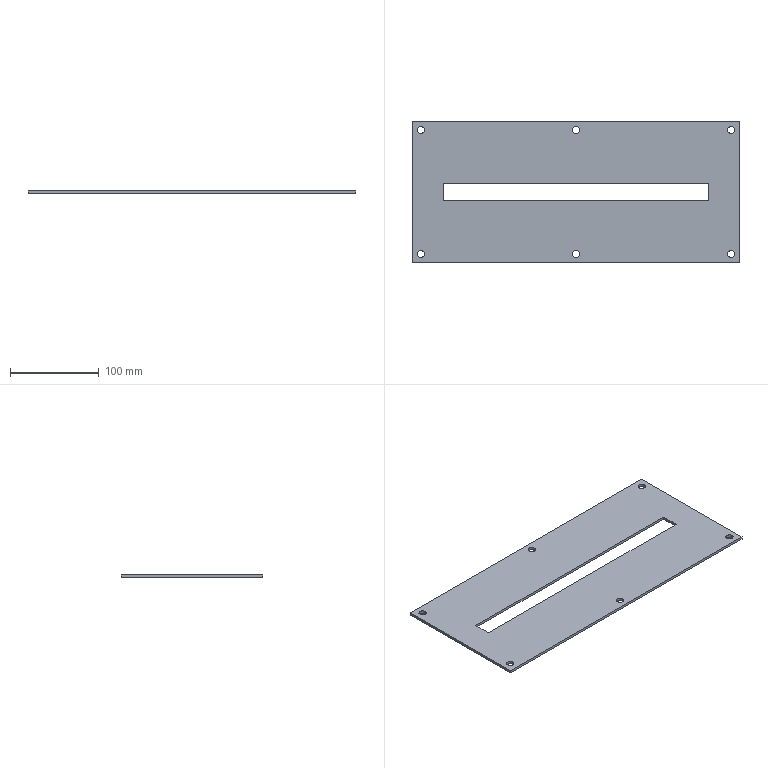Part | STEP file | SYL_0392D6J1SYL0380DJ10-1554045 | 1 solid | 22 faces | box 370 x 160 x 3 mm | volume 158695 mm3 | cylinder 12 | plane 10 | commonest cylinder face diameters 8 x12
STEP:
#1=CARTESIAN_POINT('',(179.,-70.,-3.));
#2=VERTEX_POINT('',#1);
#3=CARTESIAN_POINT('',(171.,-70.,-3.));
#4=VERTEX_POINT('',#3);
#5=CARTESIAN_POINT('',(175.,-70.,-3.));
#6=DIRECTION('',(0.,0.,1.));
#7=DIRECTION('',(1.,0.,0.));
#8=AXIS2_PLACEMENT_3D('',#5,#6,#7);
#9=CIRCLE('',#8,4.);
#10=EDGE_CURVE('',#2,#4,#9,.T.);
#11=ORIENTED_EDGE('',*,*,#10,.F.);
#12=CARTESIAN_POINT('',(179.,-70.,0.));
#13=VERTEX_POINT('',#12);
#14=CARTESIAN_POINT('',(179.,-70.,0.));
#15=DIRECTION('',(0.,0.,-1.));
#16=VECTOR('',#15,1000.);
#17=LINE('',#14,#16);
#18=EDGE_CURVE('',#13,#2,#17,.T.);
#19=ORIENTED_EDGE('',*,*,#18,.F.);
#20=CARTESIAN_POINT('',(171.,-70.,0.));
#21=VERTEX_POINT('',#20);
#22=CARTESIAN_POINT('',(175.,-70.,0.));
#23=DIRECTION('',(0.,0.,-1.));
#24=DIRECTION('',(-1.,0.,0.));
#25=AXIS2_PLACEMENT_3D('',#22,#23,#24);
#26=CIRCLE('',#25,4.);
#27=EDGE_CURVE('',#21,#13,#26,.T.);
#28=ORIENTED_EDGE('',*,*,#27,.F.);
#29=CARTESIAN_POINT('',(171.,-70.,0.));
#30=DIRECTION('',(0.,0.,-1.));
#31=VECTOR('',#30,1000.);
#32=LINE('',#29,#31);
#33=EDGE_CURVE('',#21,#4,#32,.T.);
#34=ORIENTED_EDGE('',*,*,#33,.T.);
#35=EDGE_LOOP('',(#11,#19,#28,#34));
#36=FACE_OUTER_BOUND('',#35,.T.);
#37=CARTESIAN_POINT('',(175.,-70.,-1.5));
#38=DIRECTION('',(0.,0.,1.));
#39=DIRECTION('',(1.,0.,0.));
#40=AXIS2_PLACEMENT_3D('',#37,#38,#39);
#41=CYLINDRICAL_SURFACE('',#40,4.);
#42=ADVANCED_FACE('',(#36),#41,.F.);
#43=ORIENTED_EDGE('',*,*,#33,.F.);
#44=CARTESIAN_POINT('',(175.,-70.,0.));
#45=DIRECTION('',(0.,0.,-1.));
#46=DIRECTION('',(1.,0.,0.));
#47=AXIS2_PLACEMENT_3D('',#44,#45,#46);
#48=CIRCLE('',#47,4.);
#49=EDGE_CURVE('',#13,#21,#48,.T.);
#50=ORIENTED_EDGE('',*,*,#49,.F.);
#51=ORIENTED_EDGE('',*,*,#18,.T.);
#52=CARTESIAN_POINT('',(175.,-70.,-3.));
#53=DIRECTION('',(0.,0.,1.));
#54=DIRECTION('',(-1.,0.,0.));
#55=AXIS2_PLACEMENT_3D('',#52,#53,#54);
#56=CIRCLE('',#55,4.);
#57=EDGE_CURVE('',#4,#2,#56,.T.);
#58=ORIENTED_EDGE('',*,*,#57,.F.);
#59=EDGE_LOOP('',(#43,#50,#51,#58));
#60=FACE_OUTER_BOUND('',#59,.T.);
#61=CARTESIAN_POINT('',(175.,-70.,-1.5));
#62=DIRECTION('',(0.,0.,1.));
#63=DIRECTION('',(1.,0.,0.));
#64=AXIS2_PLACEMENT_3D('',#61,#62,#63);
#65=CYLINDRICAL_SURFACE('',#64,4.);
#66=ADVANCED_FACE('',(#60),#65,.F.);
#67=CARTESIAN_POINT('',(4.,-70.,-3.));
#68=VERTEX_POINT('',#67);
#69=CARTESIAN_POINT('',(-4.,-70.,-3.));
#70=VERTEX_POINT('',#69);
#71=CARTESIAN_POINT('',(0.,-70.,-3.));
#72=DIRECTION('',(0.,0.,1.));
#73=DIRECTION('',(1.,0.,0.));
#74=AXIS2_PLACEMENT_3D('',#71,#72,#73);
#75=CIRCLE('',#74,4.);
#76=EDGE_CURVE('',#68,#70,#75,.T.);
#77=ORIENTED_EDGE('',*,*,#76,.F.);
#78=CARTESIAN_POINT('',(4.,-70.,0.));
#79=VERTEX_POINT('',#78);
#80=CARTESIAN_POINT('',(4.,-70.,0.));
#81=DIRECTION('',(0.,0.,-1.));
#82=VECTOR('',#81,1000.);
#83=LINE('',#80,#82);
#84=EDGE_CURVE('',#79,#68,#83,.T.);
#85=ORIENTED_EDGE('',*,*,#84,.F.);
#86=CARTESIAN_POINT('',(-4.,-70.,0.));
#87=VERTEX_POINT('',#86);
#88=CARTESIAN_POINT('',(0.,-70.,0.));
#89=DIRECTION('',(0.,0.,-1.));
#90=DIRECTION('',(-1.,0.,0.));
#91=AXIS2_PLACEMENT_3D('',#88,#89,#90);
#92=CIRCLE('',#91,4.);
#93=EDGE_CURVE('',#87,#79,#92,.T.);
#94=ORIENTED_EDGE('',*,*,#93,.F.);
#95=CARTESIAN_POINT('',(-4.,-70.,0.));
#96=DIRECTION('',(0.,0.,-1.));
#97=VECTOR('',#96,1000.);
#98=LINE('',#95,#97);
#99=EDGE_CURVE('',#87,#70,#98,.T.);
#100=ORIENTED_EDGE('',*,*,#99,.T.);
#101=EDGE_LOOP('',(#77,#85,#94,#100));
#102=FACE_OUTER_BOUND('',#101,.T.);
#103=CARTESIAN_POINT('',(0.,-70.,-1.5));
#104=DIRECTION('',(0.,0.,1.));
#105=DIRECTION('',(1.,0.,0.));
#106=AXIS2_PLACEMENT_3D('',#103,#104,#105);
#107=CYLINDRICAL_SURFACE('',#106,4.);
#108=ADVANCED_FACE('',(#102),#107,.F.);
#109=ORIENTED_EDGE('',*,*,#99,.F.);
#110=CARTESIAN_POINT('',(0.,-70.,0.));
#111=DIRECTION('',(0.,0.,-1.));
#112=DIRECTION('',(1.,0.,0.));
#113=AXIS2_PLACEMENT_3D('',#110,#111,#112);
#114=CIRCLE('',#113,4.);
#115=EDGE_CURVE('',#79,#87,#114,.T.);
#116=ORIENTED_EDGE('',*,*,#115,.F.);
#117=ORIENTED_EDGE('',*,*,#84,.T.);
#118=CARTESIAN_POINT('',(0.,-70.,-3.));
#119=DIRECTION('',(0.,0.,1.));
#120=DIRECTION('',(-1.,0.,0.));
#121=AXIS2_PLACEMENT_3D('',#118,#119,#120);
#122=CIRCLE('',#121,4.);
#123=EDGE_CURVE('',#70,#68,#122,.T.);
#124=ORIENTED_EDGE('',*,*,#123,.F.);
#125=EDGE_LOOP('',(#109,#116,#117,#124));
#126=FACE_OUTER_BOUND('',#125,.T.);
#127=CARTESIAN_POINT('',(0.,-70.,-1.5));
#128=DIRECTION('',(0.,0.,1.));
#129=DIRECTION('',(1.,0.,0.));
#130=AXIS2_PLACEMENT_3D('',#127,#128,#129);
#131=CYLINDRICAL_SURFACE('',#130,4.);
#132=ADVANCED_FACE('',(#126),#131,.F.);
#133=CARTESIAN_POINT('',(-171.,-70.,-3.));
#134=VERTEX_POINT('',#133);
#135=CARTESIAN_POINT('',(-179.,-70.,-3.));
#136=VERTEX_POINT('',#135);
#137=CARTESIAN_POINT('',(-175.,-70.,-3.));
#138=DIRECTION('',(0.,0.,1.));
#139=DIRECTION('',(1.,0.,0.));
#140=AXIS2_PLACEMENT_3D('',#137,#138,#139);
#141=CIRCLE('',#140,4.);
#142=EDGE_CURVE('',#134,#136,#141,.T.);
#143=ORIENTED_EDGE('',*,*,#142,.F.);
#144=CARTESIAN_POINT('',(-171.,-70.,0.));
#145=VERTEX_POINT('',#144);
#146=CARTESIAN_POINT('',(-171.,-70.,0.));
#147=DIRECTION('',(0.,0.,-1.));
#148=VECTOR('',#147,1000.);
#149=LINE('',#146,#148);
#150=EDGE_CURVE('',#145,#134,#149,.T.);
#151=ORIENTED_EDGE('',*,*,#150,.F.);
#152=CARTESIAN_POINT('',(-179.,-70.,0.));
#153=VERTEX_POINT('',#152);
#154=CARTESIAN_POINT('',(-175.,-70.,0.));
#155=DIRECTION('',(0.,0.,-1.));
#156=DIRECTION('',(-1.,0.,0.));
#157=AXIS2_PLACEMENT_3D('',#154,#155,#156);
#158=CIRCLE('',#157,4.);
#159=EDGE_CURVE('',#153,#145,#158,.T.);
#160=ORIENTED_EDGE('',*,*,#159,.F.);
#161=CARTESIAN_POINT('',(-179.,-70.,0.));
#162=DIRECTION('',(0.,0.,-1.));
#163=VECTOR('',#162,1000.);
#164=LINE('',#161,#163);
#165=EDGE_CURVE('',#153,#136,#164,.T.);
#166=ORIENTED_EDGE('',*,*,#165,.T.);
#167=EDGE_LOOP('',(#143,#151,#160,#166));
#168=FACE_OUTER_BOUND('',#167,.T.);
#169=CARTESIAN_POINT('',(-175.,-70.,-1.5));
#170=DIRECTION('',(0.,0.,1.));
#171=DIRECTION('',(1.,0.,0.));
#172=AXIS2_PLACEMENT_3D('',#169,#170,#171);
#173=CYLINDRICAL_SURFACE('',#172,4.);
#174=ADVANCED_FACE('',(#168),#173,.F.);
#175=ORIENTED_EDGE('',*,*,#165,.F.);
#176=CARTESIAN_POINT('',(-175.,-70.,0.));
#177=DIRECTION('',(0.,0.,-1.));
#178=DIRECTION('',(1.,0.,0.));
#179=AXIS2_PLACEMENT_3D('',#176,#177,#178);
#180=CIRCLE('',#179,4.);
#181=EDGE_CURVE('',#145,#153,#180,.T.);
#182=ORIENTED_EDGE('',*,*,#181,.F.);
#183=ORIENTED_EDGE('',*,*,#150,.T.);
#184=CARTESIAN_POINT('',(-175.,-70.,-3.));
#185=DIRECTION('',(0.,0.,1.));
#186=DIRECTION('',(-1.,0.,0.));
#187=AXIS2_PLACEMENT_3D('',#184,#185,#186);
#188=CIRCLE('',#187,4.);
#189=EDGE_CURVE('',#136,#134,#188,.T.);
#190=ORIENTED_EDGE('',*,*,#189,.F.);
#191=EDGE_LOOP('',(#175,#182,#183,#190));
#192=FACE_OUTER_BOUND('',#191,.T.);
#193=CARTESIAN_POINT('',(-175.,-70.,-1.5));
#194=DIRECTION('',(0.,0.,1.));
#195=DIRECTION('',(1.,0.,0.));
#196=AXIS2_PLACEMENT_3D('',#193,#194,#195);
#197=CYLINDRICAL_SURFACE('',#196,4.);
#198=ADVANCED_FACE('',(#192),#197,.F.);
#199=CARTESIAN_POINT('',(179.,70.,-3.));
#200=VERTEX_POINT('',#199);
#201=CARTESIAN_POINT('',(171.,70.,-3.));
#202=VERTEX_POINT('',#201);
#203=CARTESIAN_POINT('',(175.,70.,-3.));
#204=DIRECTION('',(0.,0.,1.));
#205=DIRECTION('',(1.,0.,0.));
#206=AXIS2_PLACEMENT_3D('',#203,#204,#205);
#207=CIRCLE('',#206,4.);
#208=EDGE_CURVE('',#200,#202,#207,.T.);
#209=ORIENTED_EDGE('',*,*,#208,.F.);
#210=CARTESIAN_POINT('',(179.,70.,0.));
#211=VERTEX_POINT('',#210);
#212=CARTESIAN_POINT('',(179.,70.,0.));
#213=DIRECTION('',(0.,0.,-1.));
#214=VECTOR('',#213,1000.);
#215=LINE('',#212,#214);
#216=EDGE_CURVE('',#211,#200,#215,.T.);
#217=ORIENTED_EDGE('',*,*,#216,.F.);
#218=CARTESIAN_POINT('',(171.,70.,0.));
#219=VERTEX_POINT('',#218);
#220=CARTESIAN_POINT('',(175.,70.,0.));
#221=DIRECTION('',(0.,0.,-1.));
#222=DIRECTION('',(-1.,0.,0.));
#223=AXIS2_PLACEMENT_3D('',#220,#221,#222);
#224=CIRCLE('',#223,4.);
#225=EDGE_CURVE('',#219,#211,#224,.T.);
#226=ORIENTED_EDGE('',*,*,#225,.F.);
#227=CARTESIAN_POINT('',(171.,70.,0.));
#228=DIRECTION('',(0.,0.,-1.));
#229=VECTOR('',#228,1000.);
#230=LINE('',#227,#229);
#231=EDGE_CURVE('',#219,#202,#230,.T.);
#232=ORIENTED_EDGE('',*,*,#231,.T.);
#233=EDGE_LOOP('',(#209,#217,#226,#232));
#234=FACE_OUTER_BOUND('',#233,.T.);
#235=CARTESIAN_POINT('',(175.,70.,-1.5));
#236=DIRECTION('',(0.,0.,1.));
#237=DIRECTION('',(1.,0.,0.));
#238=AXIS2_PLACEMENT_3D('',#235,#236,#237);
#239=CYLINDRICAL_SURFACE('',#238,4.);
#240=ADVANCED_FACE('',(#234),#239,.F.);
#241=ORIENTED_EDGE('',*,*,#231,.F.);
#242=CARTESIAN_POINT('',(175.,70.,0.));
#243=DIRECTION('',(0.,0.,-1.));
#244=DIRECTION('',(1.,0.,0.));
#245=AXIS2_PLACEMENT_3D('',#242,#243,#244);
#246=CIRCLE('',#245,4.);
#247=EDGE_CURVE('',#211,#219,#246,.T.);
#248=ORIENTED_EDGE('',*,*,#247,.F.);
#249=ORIENTED_EDGE('',*,*,#216,.T.);
#250=CARTESIAN_POINT('',(175.,70.,-3.));
#251=DIRECTION('',(0.,0.,1.));
#252=DIRECTION('',(-1.,0.,0.));
#253=AXIS2_PLACEMENT_3D('',#250,#251,#252);
#254=CIRCLE('',#253,4.);
#255=EDGE_CURVE('',#202,#200,#254,.T.);
#256=ORIENTED_EDGE('',*,*,#255,.F.);
#257=EDGE_LOOP('',(#241,#248,#249,#256));
#258=FACE_OUTER_BOUND('',#257,.T.);
#259=CARTESIAN_POINT('',(175.,70.,-1.5));
#260=DIRECTION('',(0.,0.,1.));
#261=DIRECTION('',(1.,0.,0.));
#262=AXIS2_PLACEMENT_3D('',#259,#260,#261);
#263=CYLINDRICAL_SURFACE('',#262,4.);
#264=ADVANCED_FACE('',(#258),#263,.F.);
#265=CARTESIAN_POINT('',(4.,70.,-3.));
#266=VERTEX_POINT('',#265);
#267=CARTESIAN_POINT('',(-4.,70.,-3.));
#268=VERTEX_POINT('',#267);
#269=CARTESIAN_POINT('',(0.,70.,-3.));
#270=DIRECTION('',(0.,0.,1.));
#271=DIRECTION('',(1.,0.,0.));
#272=AXIS2_PLACEMENT_3D('',#269,#270,#271);
#273=CIRCLE('',#272,4.);
#274=EDGE_CURVE('',#266,#268,#273,.T.);
#275=ORIENTED_EDGE('',*,*,#274,.F.);
#276=CARTESIAN_POINT('',(4.,70.,0.));
#277=VERTEX_POINT('',#276);
#278=CARTESIAN_POINT('',(4.,70.,0.));
#279=DIRECTION('',(0.,0.,-1.));
#280=VECTOR('',#279,1000.);
#281=LINE('',#278,#280);
#282=EDGE_CURVE('',#277,#266,#281,.T.);
#283=ORIENTED_EDGE('',*,*,#282,.F.);
#284=CARTESIAN_POINT('',(-4.,70.,0.));
#285=VERTEX_POINT('',#284);
#286=CARTESIAN_POINT('',(0.,70.,0.));
#287=DIRECTION('',(0.,0.,-1.));
#288=DIRECTION('',(-1.,0.,0.));
#289=AXIS2_PLACEMENT_3D('',#286,#287,#288);
#290=CIRCLE('',#289,4.);
#291=EDGE_CURVE('',#285,#277,#290,.T.);
#292=ORIENTED_EDGE('',*,*,#291,.F.);
#293=CARTESIAN_POINT('',(-4.,70.,0.));
#294=DIRECTION('',(0.,0.,-1.));
#295=VECTOR('',#294,1000.);
#296=LINE('',#293,#295);
#297=EDGE_CURVE('',#285,#268,#296,.T.);
#298=ORIENTED_EDGE('',*,*,#297,.T.);
#299=EDGE_LOOP('',(#275,#283,#292,#298));
#300=FACE_OUTER_BOUND('',#299,.T.);
#301=CARTESIAN_POINT('',(0.,70.,-1.5));
#302=DIRECTION('',(0.,0.,1.));
#303=DIRECTION('',(1.,0.,0.));
#304=AXIS2_PLACEMENT_3D('',#301,#302,#303);
#305=CYLINDRICAL_SURFACE('',#304,4.);
#306=ADVANCED_FACE('',(#300),#305,.F.);
#307=ORIENTED_EDGE('',*,*,#297,.F.);
#308=CARTESIAN_POINT('',(0.,70.,0.));
#309=DIRECTION('',(0.,0.,-1.));
#310=DIRECTION('',(1.,0.,0.));
#311=AXIS2_PLACEMENT_3D('',#308,#309,#310);
#312=CIRCLE('',#311,4.);
#313=EDGE_CURVE('',#277,#285,#312,.T.);
#314=ORIENTED_EDGE('',*,*,#313,.F.);
#315=ORIENTED_EDGE('',*,*,#282,.T.);
#316=CARTESIAN_POINT('',(0.,70.,-3.));
#317=DIRECTION('',(0.,0.,1.));
#318=DIRECTION('',(-1.,0.,0.));
#319=AXIS2_PLACEMENT_3D('',#316,#317,#318);
#320=CIRCLE('',#319,4.);
#321=EDGE_CURVE('',#268,#266,#320,.T.);
#322=ORIENTED_EDGE('',*,*,#321,.F.);
#323=EDGE_LOOP('',(#307,#314,#315,#322));
#324=FACE_OUTER_BOUND('',#323,.T.);
#325=CARTESIAN_POINT('',(0.,70.,-1.5));
#326=DIRECTION('',(0.,0.,1.));
#327=DIRECTION('',(1.,0.,0.));
#328=AXIS2_PLACEMENT_3D('',#325,#326,#327);
#329=CYLINDRICAL_SURFACE('',#328,4.);
#330=ADVANCED_FACE('',(#324),#329,.F.);
#331=CARTESIAN_POINT('',(-171.,70.,-3.));
#332=VERTEX_POINT('',#331);
#333=CARTESIAN_POINT('',(-179.,70.,-3.));
#334=VERTEX_POINT('',#333);
#335=CARTESIAN_POINT('',(-175.,70.,-3.));
#336=DIRECTION('',(0.,0.,1.));
#337=DIRECTION('',(1.,0.,0.));
#338=AXIS2_PLACEMENT_3D('',#335,#336,#337);
#339=CIRCLE('',#338,4.);
#340=EDGE_CURVE('',#332,#334,#339,.T.);
#341=ORIENTED_EDGE('',*,*,#340,.F.);
#342=CARTESIAN_POINT('',(-171.,70.,0.));
#343=VERTEX_POINT('',#342);
#344=CARTESIAN_POINT('',(-171.,70.,0.));
#345=DIRECTION('',(0.,0.,-1.));
#346=VECTOR('',#345,1000.);
#347=LINE('',#344,#346);
#348=EDGE_CURVE('',#343,#332,#347,.T.);
#349=ORIENTED_EDGE('',*,*,#348,.F.);
#350=CARTESIAN_POINT('',(-179.,70.,0.));
#351=VERTEX_POINT('',#350);
#352=CARTESIAN_POINT('',(-175.,70.,0.));
#353=DIRECTION('',(0.,0.,-1.));
#354=DIRECTION('',(-1.,0.,0.));
#355=AXIS2_PLACEMENT_3D('',#352,#353,#354);
#356=CIRCLE('',#355,4.);
#357=EDGE_CURVE('',#351,#343,#356,.T.);
#358=ORIENTED_EDGE('',*,*,#357,.F.);
#359=CARTESIAN_POINT('',(-179.,70.,0.));
#360=DIRECTION('',(0.,0.,-1.));
#361=VECTOR('',#360,1000.);
#362=LINE('',#359,#361);
#363=EDGE_CURVE('',#351,#334,#362,.T.);
#364=ORIENTED_EDGE('',*,*,#363,.T.);
#365=EDGE_LOOP('',(#341,#349,#358,#364));
#366=FACE_OUTER_BOUND('',#365,.T.);
#367=CARTESIAN_POINT('',(-175.,70.,-1.5));
#368=DIRECTION('',(0.,0.,1.));
#369=DIRECTION('',(1.,0.,0.));
#370=AXIS2_PLACEMENT_3D('',#367,#368,#369);
#371=CYLINDRICAL_SURFACE('',#370,4.);
#372=ADVANCED_FACE('',(#366),#371,.F.);
#373=ORIENTED_EDGE('',*,*,#363,.F.);
#374=CARTESIAN_POINT('',(-175.,70.,0.));
#375=DIRECTION('',(0.,0.,-1.));
#376=DIRECTION('',(1.,0.,0.));
#377=AXIS2_PLACEMENT_3D('',#374,#375,#376);
#378=CIRCLE('',#377,4.);
#379=EDGE_CURVE('',#343,#351,#378,.T.);
#380=ORIENTED_EDGE('',*,*,#379,.F.);
#381=ORIENTED_EDGE('',*,*,#348,.T.);
#382=CARTESIAN_POINT('',(-175.,70.,-3.));
#383=DIRECTION('',(0.,0.,1.));
#384=DIRECTION('',(-1.,0.,0.));
#385=AXIS2_PLACEMENT_3D('',#382,#383,#384);
#386=CIRCLE('',#385,4.);
#387=EDGE_CURVE('',#334,#332,#386,.T.);
#388=ORIENTED_EDGE('',*,*,#387,.F.);
#389=EDGE_LOOP('',(#373,#380,#381,#388));
#390=FACE_OUTER_BOUND('',#389,.T.);
#391=CARTESIAN_POINT('',(-175.,70.,-1.5));
#392=DIRECTION('',(0.,0.,1.));
#393=DIRECTION('',(1.,0.,0.));
#394=AXIS2_PLACEMENT_3D('',#391,#392,#393);
#395=CYLINDRICAL_SURFACE('',#394,4.);
#396=ADVANCED_FACE('',(#390),#395,.F.);
#397=CARTESIAN_POINT('',(150.,10.,0.));
#398=VERTEX_POINT('',#397);
#399=CARTESIAN_POINT('',(-150.,10.,0.));
#400=VERTEX_POINT('',#399);
#401=CARTESIAN_POINT('',(150.,10.,0.));
#402=DIRECTION('',(-1.,0.,0.));
#403=VECTOR('',#402,1000.);
#404=LINE('',#401,#403);
#405=EDGE_CURVE('',#398,#400,#404,.T.);
#406=ORIENTED_EDGE('',*,*,#405,.F.);
#407=CARTESIAN_POINT('',(150.,-10.,0.));
#408=VERTEX_POINT('',#407);
#409=CARTESIAN_POINT('',(150.,-10.,0.));
#410=DIRECTION('',(0.,1.,0.));
#411=VECTOR('',#410,1000.);
#412=LINE('',#409,#411);
#413=EDGE_CURVE('',#408,#398,#412,.T.);
#414=ORIENTED_EDGE('',*,*,#413,.F.);
#415=CARTESIAN_POINT('',(-150.,-10.,0.));
#416=VERTEX_POINT('',#415);
#417=CARTESIAN_POINT('',(-150.,-10.,0.));
#418=DIRECTION('',(1.,0.,0.));
#419=VECTOR('',#418,1000.);
#420=LINE('',#417,#419);
#421=EDGE_CURVE('',#416,#408,#420,.T.);
#422=ORIENTED_EDGE('',*,*,#421,.F.);
#423=CARTESIAN_POINT('',(-150.,10.,0.));
#424=DIRECTION('',(0.,-1.,0.));
#425=VECTOR('',#424,1000.);
#426=LINE('',#423,#425);
#427=EDGE_CURVE('',#400,#416,#426,.T.);
#428=ORIENTED_EDGE('',*,*,#427,.F.);
#429=EDGE_LOOP('',(#406,#414,#422,#428));
#430=FACE_BOUND('',#429,.T.);
#431=ORIENTED_EDGE('',*,*,#27,.T.);
#432=ORIENTED_EDGE('',*,*,#49,.T.);
#433=EDGE_LOOP('',(#431,#432));
#434=FACE_BOUND('',#433,.T.);
#435=ORIENTED_EDGE('',*,*,#93,.T.);
#436=ORIENTED_EDGE('',*,*,#115,.T.);
#437=EDGE_LOOP('',(#435,#436));
#438=FACE_BOUND('',#437,.T.);
#439=ORIENTED_EDGE('',*,*,#159,.T.);
#440=ORIENTED_EDGE('',*,*,#181,.T.);
#441=EDGE_LOOP('',(#439,#440));
#442=FACE_BOUND('',#441,.T.);
#443=ORIENTED_EDGE('',*,*,#225,.T.);
#444=ORIENTED_EDGE('',*,*,#247,.T.);
#445=EDGE_LOOP('',(#443,#444));
#446=FACE_BOUND('',#445,.T.);
#447=ORIENTED_EDGE('',*,*,#291,.T.);
#448=ORIENTED_EDGE('',*,*,#313,.T.);
#449=EDGE_LOOP('',(#447,#448));
#450=FACE_BOUND('',#449,.T.);
#451=ORIENTED_EDGE('',*,*,#357,.T.);
#452=ORIENTED_EDGE('',*,*,#379,.T.);
#453=EDGE_LOOP('',(#451,#452));
#454=FACE_BOUND('',#453,.T.);
#455=CARTESIAN_POINT('',(-185.,-80.,0.));
#456=VERTEX_POINT('',#455);
#457=CARTESIAN_POINT('',(-185.,80.,0.));
#458=VERTEX_POINT('',#457);
#459=CARTESIAN_POINT('',(-185.,-80.,0.));
#460=DIRECTION('',(0.,1.,0.));
#461=VECTOR('',#460,1000.);
#462=LINE('',#459,#461);
#463=EDGE_CURVE('',#456,#458,#462,.T.);
#464=ORIENTED_EDGE('',*,*,#463,.F.);
#465=CARTESIAN_POINT('',(185.,-80.,0.));
#466=VERTEX_POINT('',#465);
#467=CARTESIAN_POINT('',(185.,-80.,0.));
#468=DIRECTION('',(-1.,0.,0.));
#469=VECTOR('',#468,1000.);
#470=LINE('',#467,#469);
#471=EDGE_CURVE('',#466,#456,#470,.T.);
#472=ORIENTED_EDGE('',*,*,#471,.F.);
#473=CARTESIAN_POINT('',(185.,80.,0.));
#474=VERTEX_POINT('',#473);
#475=CARTESIAN_POINT('',(185.,80.,0.));
#476=DIRECTION('',(0.,-1.,0.));
#477=VECTOR('',#476,1000.);
#478=LINE('',#475,#477);
#479=EDGE_CURVE('',#474,#466,#478,.T.);
#480=ORIENTED_EDGE('',*,*,#479,.F.);
#481=CARTESIAN_POINT('',(-185.,80.,0.));
#482=DIRECTION('',(1.,0.,0.));
#483=VECTOR('',#482,1000.);
#484=LINE('',#481,#483);
#485=EDGE_CURVE('',#458,#474,#484,.T.);
#486=ORIENTED_EDGE('',*,*,#485,.F.);
#487=EDGE_LOOP('',(#464,#472,#480,#486));
#488=FACE_OUTER_BOUND('',#487,.T.);
#489=CARTESIAN_POINT('',(0.,0.,0.));
#490=DIRECTION('',(0.,0.,1.));
#491=DIRECTION('',(1.,0.,0.));
#492=AXIS2_PLACEMENT_3D('',#489,#490,#491);
#493=PLANE('',#492);
#494=ADVANCED_FACE('',(#430,#434,#438,#442,#446,#450,#454,#488),#493,.T.);
#495=ORIENTED_EDGE('',*,*,#471,.T.);
#496=CARTESIAN_POINT('',(-185.,-80.,-3.));
#497=VERTEX_POINT('',#496);
#498=CARTESIAN_POINT('',(-185.,-80.,0.));
#499=DIRECTION('',(0.,0.,-1.));
#500=VECTOR('',#499,1000.);
#501=LINE('',#498,#500);
#502=EDGE_CURVE('',#456,#497,#501,.T.);
#503=ORIENTED_EDGE('',*,*,#502,.T.);
#504=CARTESIAN_POINT('',(185.,-80.,-3.));
#505=VERTEX_POINT('',#504);
#506=CARTESIAN_POINT('',(185.,-80.,-3.));
#507=DIRECTION('',(-1.,0.,0.));
#508=VECTOR('',#507,1000.);
#509=LINE('',#506,#508);
#510=EDGE_CURVE('',#505,#497,#509,.T.);
#511=ORIENTED_EDGE('',*,*,#510,.F.);
#512=CARTESIAN_POINT('',(185.,-80.,-3.));
#513=DIRECTION('',(0.,0.,1.));
#514=VECTOR('',#513,1000.);
#515=LINE('',#512,#514);
#516=EDGE_CURVE('',#505,#466,#515,.T.);
#517=ORIENTED_EDGE('',*,*,#516,.T.);
#518=EDGE_LOOP('',(#495,#503,#511,#517));
#519=FACE_OUTER_BOUND('',#518,.T.);
#520=CARTESIAN_POINT('',(0.,-80.,-1.5));
#521=DIRECTION('',(0.,-1.,0.));
#522=DIRECTION('',(0.,0.,-1.));
#523=AXIS2_PLACEMENT_3D('',#520,#521,#522);
#524=PLANE('',#523);
#525=ADVANCED_FACE('',(#519),#524,.T.);
#526=ORIENTED_EDGE('',*,*,#463,.T.);
#527=CARTESIAN_POINT('',(-185.,80.,-3.));
#528=VERTEX_POINT('',#527);
#529=CARTESIAN_POINT('',(-185.,80.,-3.));
#530=DIRECTION('',(0.,0.,1.));
#531=VECTOR('',#530,1000.);
#532=LINE('',#529,#531);
#533=EDGE_CURVE('',#528,#458,#532,.T.);
#534=ORIENTED_EDGE('',*,*,#533,.F.);
#535=CARTESIAN_POINT('',(-185.,-80.,-3.));
#536=DIRECTION('',(0.,1.,0.));
#537=VECTOR('',#536,1000.);
#538=LINE('',#535,#537);
#539=EDGE_CURVE('',#497,#528,#538,.T.);
#540=ORIENTED_EDGE('',*,*,#539,.F.);
#541=ORIENTED_EDGE('',*,*,#502,.F.);
#542=EDGE_LOOP('',(#526,#534,#540,#541));
#543=FACE_OUTER_BOUND('',#542,.T.);
#544=CARTESIAN_POINT('',(-185.,0.,-1.5));
#545=DIRECTION('',(-1.,0.,0.));
#546=DIRECTION('',(0.,0.,1.));
#547=AXIS2_PLACEMENT_3D('',#544,#545,#546);
#548=PLANE('',#547);
#549=ADVANCED_FACE('',(#543),#548,.T.);
#550=ORIENTED_EDGE('',*,*,#485,.T.);
#551=CARTESIAN_POINT('',(185.,80.,-3.));
#552=VERTEX_POINT('',#551);
#553=CARTESIAN_POINT('',(185.,80.,-3.));
#554=DIRECTION('',(0.,0.,1.));
#555=VECTOR('',#554,1000.);
#556=LINE('',#553,#555);
#557=EDGE_CURVE('',#552,#474,#556,.T.);
#558=ORIENTED_EDGE('',*,*,#557,.F.);
#559=CARTESIAN_POINT('',(-185.,80.,-3.));
#560=DIRECTION('',(1.,0.,0.));
#561=VECTOR('',#560,1000.);
#562=LINE('',#559,#561);
#563=EDGE_CURVE('',#528,#552,#562,.T.);
#564=ORIENTED_EDGE('',*,*,#563,.F.);
#565=ORIENTED_EDGE('',*,*,#533,.T.);
#566=EDGE_LOOP('',(#550,#558,#564,#565));
#567=FACE_OUTER_BOUND('',#566,.T.);
#568=CARTESIAN_POINT('',(0.,80.,-1.5));
#569=DIRECTION('',(0.,1.,0.));
#570=DIRECTION('',(1.,0.,0.));
#571=AXIS2_PLACEMENT_3D('',#568,#569,#570);
#572=PLANE('',#571);
#573=ADVANCED_FACE('',(#567),#572,.T.);
#574=ORIENTED_EDGE('',*,*,#479,.T.);
#575=ORIENTED_EDGE('',*,*,#516,.F.);
#576=CARTESIAN_POINT('',(185.,80.,-3.));
#577=DIRECTION('',(0.,-1.,0.));
#578=VECTOR('',#577,1000.);
#579=LINE('',#576,#578);
#580=EDGE_CURVE('',#552,#505,#579,.T.);
#581=ORIENTED_EDGE('',*,*,#580,.F.);
#582=ORIENTED_EDGE('',*,*,#557,.T.);
#583=EDGE_LOOP('',(#574,#575,#581,#582));
#584=FACE_OUTER_BOUND('',#583,.T.);
#585=CARTESIAN_POINT('',(185.,0.,-1.5));
#586=DIRECTION('',(1.,0.,0.));
#587=DIRECTION('',(0.,1.,0.));
#588=AXIS2_PLACEMENT_3D('',#585,#586,#587);
#589=PLANE('',#588);
#590=ADVANCED_FACE('',(#584),#589,.T.);
#591=CARTESIAN_POINT('',(150.,-10.,-3.));
#592=VERTEX_POINT('',#591);
#593=CARTESIAN_POINT('',(150.,10.,-3.));
#594=VERTEX_POINT('',#593);
#595=CARTESIAN_POINT('',(150.,-10.,-3.));
#596=DIRECTION('',(0.,1.,0.));
#597=VECTOR('',#596,1000.);
#598=LINE('',#595,#597);
#599=EDGE_CURVE('',#592,#594,#598,.T.);
#600=ORIENTED_EDGE('',*,*,#599,.T.);
#601=CARTESIAN_POINT('',(-150.,10.,-3.));
#602=VERTEX_POINT('',#601);
#603=CARTESIAN_POINT('',(150.,10.,-3.));
#604=DIRECTION('',(-1.,0.,0.));
#605=VECTOR('',#604,1000.);
#606=LINE('',#603,#605);
#607=EDGE_CURVE('',#594,#602,#606,.T.);
#608=ORIENTED_EDGE('',*,*,#607,.T.);
#609=CARTESIAN_POINT('',(-150.,-10.,-3.));
#610=VERTEX_POINT('',#609);
#611=CARTESIAN_POINT('',(-150.,10.,-3.));
#612=DIRECTION('',(0.,-1.,0.));
#613=VECTOR('',#612,1000.);
#614=LINE('',#611,#613);
#615=EDGE_CURVE('',#602,#610,#614,.T.);
#616=ORIENTED_EDGE('',*,*,#615,.T.);
#617=CARTESIAN_POINT('',(-150.,-10.,-3.));
#618=DIRECTION('',(1.,0.,0.));
#619=VECTOR('',#618,1000.);
#620=LINE('',#617,#619);
#621=EDGE_CURVE('',#610,#592,#620,.T.);
#622=ORIENTED_EDGE('',*,*,#621,.T.);
#623=EDGE_LOOP('',(#600,#608,#616,#622));
#624=FACE_BOUND('',#623,.T.);
#625=ORIENTED_EDGE('',*,*,#57,.T.);
#626=ORIENTED_EDGE('',*,*,#10,.T.);
#627=EDGE_LOOP('',(#625,#626));
#628=FACE_BOUND('',#627,.T.);
#629=ORIENTED_EDGE('',*,*,#123,.T.);
#630=ORIENTED_EDGE('',*,*,#76,.T.);
#631=EDGE_LOOP('',(#629,#630));
#632=FACE_BOUND('',#631,.T.);
#633=ORIENTED_EDGE('',*,*,#189,.T.);
#634=ORIENTED_EDGE('',*,*,#142,.T.);
#635=EDGE_LOOP('',(#633,#634));
#636=FACE_BOUND('',#635,.T.);
#637=ORIENTED_EDGE('',*,*,#255,.T.);
#638=ORIENTED_EDGE('',*,*,#208,.T.);
#639=EDGE_LOOP('',(#637,#638));
#640=FACE_BOUND('',#639,.T.);
#641=ORIENTED_EDGE('',*,*,#321,.T.);
#642=ORIENTED_EDGE('',*,*,#274,.T.);
#643=EDGE_LOOP('',(#641,#642));
#644=FACE_BOUND('',#643,.T.);
#645=ORIENTED_EDGE('',*,*,#387,.T.);
#646=ORIENTED_EDGE('',*,*,#340,.T.);
#647=EDGE_LOOP('',(#645,#646));
#648=FACE_BOUND('',#647,.T.);
#649=ORIENTED_EDGE('',*,*,#510,.T.);
#650=ORIENTED_EDGE('',*,*,#539,.T.);
#651=ORIENTED_EDGE('',*,*,#563,.T.);
#652=ORIENTED_EDGE('',*,*,#580,.T.);
#653=EDGE_LOOP('',(#649,#650,#651,#652));
#654=FACE_OUTER_BOUND('',#653,.T.);
#655=CARTESIAN_POINT('',(0.,0.,-3.));
#656=DIRECTION('',(0.,0.,1.));
#657=DIRECTION('',(1.,0.,0.));
#658=AXIS2_PLACEMENT_3D('',#655,#656,#657);
#659=PLANE('',#658);
#660=ADVANCED_FACE('',(#624,#628,#632,#636,#640,#644,#648,#654),#659,.F.);
#661=ORIENTED_EDGE('',*,*,#421,.T.);
#662=CARTESIAN_POINT('',(150.,-10.,-3.));
#663=DIRECTION('',(0.,0.,1.));
#664=VECTOR('',#663,1000.);
#665=LINE('',#662,#664);
#666=EDGE_CURVE('',#592,#408,#665,.T.);
#667=ORIENTED_EDGE('',*,*,#666,.F.);
#668=ORIENTED_EDGE('',*,*,#621,.F.);
#669=CARTESIAN_POINT('',(-150.,-10.,-3.));
#670=DIRECTION('',(0.,0.,1.));
#671=VECTOR('',#670,1000.);
#672=LINE('',#669,#671);
#673=EDGE_CURVE('',#610,#416,#672,.T.);
#674=ORIENTED_EDGE('',*,*,#673,.T.);
#675=EDGE_LOOP('',(#661,#667,#668,#674));
#676=FACE_OUTER_BOUND('',#675,.T.);
#677=CARTESIAN_POINT('',(0.,-10.,-1.5));
#678=DIRECTION('',(0.,1.,0.));
#679=DIRECTION('',(1.,0.,0.));
#680=AXIS2_PLACEMENT_3D('',#677,#678,#679);
#681=PLANE('',#680);
#682=ADVANCED_FACE('',(#676),#681,.T.);
#683=ORIENTED_EDGE('',*,*,#413,.T.);
#684=CARTESIAN_POINT('',(150.,10.,0.));
#685=DIRECTION('',(0.,0.,-1.));
#686=VECTOR('',#685,1000.);
#687=LINE('',#684,#686);
#688=EDGE_CURVE('',#398,#594,#687,.T.);
#689=ORIENTED_EDGE('',*,*,#688,.T.);
#690=ORIENTED_EDGE('',*,*,#599,.F.);
#691=ORIENTED_EDGE('',*,*,#666,.T.);
#692=EDGE_LOOP('',(#683,#689,#690,#691));
#693=FACE_OUTER_BOUND('',#692,.T.);
#694=CARTESIAN_POINT('',(150.,0.,-1.5));
#695=DIRECTION('',(-1.,0.,0.));
#696=DIRECTION('',(0.,0.,1.));
#697=AXIS2_PLACEMENT_3D('',#694,#695,#696);
#698=PLANE('',#697);
#699=ADVANCED_FACE('',(#693),#698,.T.);
#700=ORIENTED_EDGE('',*,*,#405,.T.);
#701=CARTESIAN_POINT('',(-150.,10.,-3.));
#702=DIRECTION('',(0.,0.,1.));
#703=VECTOR('',#702,1000.);
#704=LINE('',#701,#703);
#705=EDGE_CURVE('',#602,#400,#704,.T.);
#706=ORIENTED_EDGE('',*,*,#705,.F.);
#707=ORIENTED_EDGE('',*,*,#607,.F.);
#708=ORIENTED_EDGE('',*,*,#688,.F.);
#709=EDGE_LOOP('',(#700,#706,#707,#708));
#710=FACE_OUTER_BOUND('',#709,.T.);
#711=CARTESIAN_POINT('',(0.,10.,-1.5));
#712=DIRECTION('',(0.,-1.,0.));
#713=DIRECTION('',(0.,0.,-1.));
#714=AXIS2_PLACEMENT_3D('',#711,#712,#713);
#715=PLANE('',#714);
#716=ADVANCED_FACE('',(#710),#715,.T.);
#717=ORIENTED_EDGE('',*,*,#427,.T.);
#718=ORIENTED_EDGE('',*,*,#673,.F.);
#719=ORIENTED_EDGE('',*,*,#615,.F.);
#720=ORIENTED_EDGE('',*,*,#705,.T.);
#721=EDGE_LOOP('',(#717,#718,#719,#720));
#722=FACE_OUTER_BOUND('',#721,.T.);
#723=CARTESIAN_POINT('',(-150.,0.,-1.5));
#724=DIRECTION('',(1.,0.,0.));
#725=DIRECTION('',(0.,1.,0.));
#726=AXIS2_PLACEMENT_3D('',#723,#724,#725);
#727=PLANE('',#726);
#728=ADVANCED_FACE('',(#722),#727,.T.);
#729=CLOSED_SHELL('',(#42,#66,#108,#132,#174,#198,#240,#264,#306,#330,#372,#396,#494,#525,#549,#573,#590,#660,#682,#699,#716,#728));
#730=MANIFOLD_SOLID_BREP('',#729);
#731=CARTESIAN_POINT('',(0.,0.,0.));
#732=DIRECTION('',(0.,0.,1.));
#733=DIRECTION('',(1.,0.,0.));
#734=AXIS2_PLACEMENT_3D('',#731,#732,#733);
#735=(LENGTH_UNIT()NAMED_UNIT(*)SI_UNIT(.MILLI.,.METRE.));
#736=UNCERTAINTY_MEASURE_WITH_UNIT(LENGTH_MEASURE(0.00001),#735,'','');
#737=(NAMED_UNIT(*)PLANE_ANGLE_UNIT()SI_UNIT($,.RADIAN.));
#738=(NAMED_UNIT(*)SI_UNIT($,.STERADIAN.)SOLID_ANGLE_UNIT());
#739=(GEOMETRIC_REPRESENTATION_CONTEXT(3)GLOBAL_UNCERTAINTY_ASSIGNED_CONTEXT((#736))GLOBAL_UNIT_ASSIGNED_CONTEXT((#735,#737,#738))REPRESENTATION_CONTEXT('',''));
#740=ADVANCED_BREP_SHAPE_REPRESENTATION('',(#730,#734),#739);